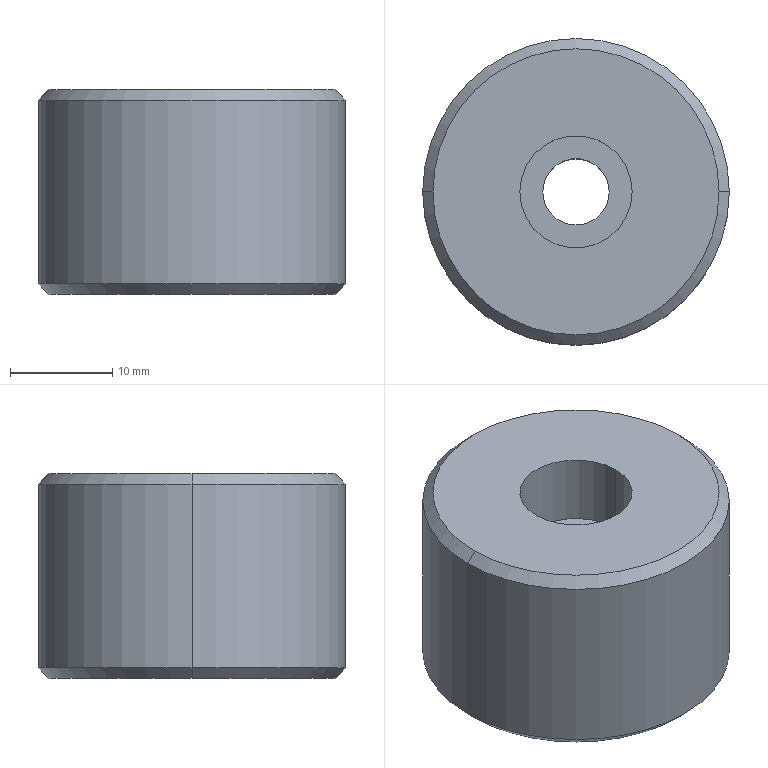Part | Creo | 1 solid | 13 faces | box 30 x 30 x 20 mm | volume 12948 mm3 | cylinder 6 | cone 4 | plane 3 | commonest cylinder face diameters 6.5 x2 11 x2 30 x2
STEP:
#1=CARTESIAN_POINT('',(-36.,235.,-210.5));
#2=VERTEX_POINT('',#1);
#3=CARTESIAN_POINT('',(-64.,235.,-210.5));
#4=VERTEX_POINT('',#3);
#5=CARTESIAN_POINT('',(-50.,235.,-210.5));
#6=DIRECTION('',(0.,0.,1.));
#7=DIRECTION('',(1.,0.,0.));
#8=AXIS2_PLACEMENT_3D('',#5,#6,#7);
#9=CIRCLE('',#8,14.);
#10=EDGE_CURVE('',#2,#4,#9,.T.);
#11=ORIENTED_EDGE('',*,*,#10,.F.);
#12=CARTESIAN_POINT('',(-50.,235.,-210.5));
#13=DIRECTION('',(0.,0.,1.));
#14=DIRECTION('',(-1.,0.,0.));
#15=AXIS2_PLACEMENT_3D('',#12,#13,#14);
#16=CIRCLE('',#15,14.);
#17=EDGE_CURVE('',#4,#2,#16,.T.);
#18=ORIENTED_EDGE('',*,*,#17,.F.);
#19=EDGE_LOOP('',(#11,#18));
#20=FACE_OUTER_BOUND('',#19,.F.);
#21=CARTESIAN_POINT('',(-55.5,235.,-210.5));
#22=VERTEX_POINT('',#21);
#23=CARTESIAN_POINT('',(-44.5,235.,-210.5));
#24=VERTEX_POINT('',#23);
#25=CARTESIAN_POINT('',(-50.,235.,-210.5));
#26=DIRECTION('',(0.,0.,-1.));
#27=DIRECTION('',(-1.,0.,0.));
#28=AXIS2_PLACEMENT_3D('',#25,#26,#27);
#29=CIRCLE('',#28,5.5);
#30=EDGE_CURVE('',#22,#24,#29,.T.);
#31=ORIENTED_EDGE('',*,*,#30,.F.);
#32=CARTESIAN_POINT('',(-50.,235.,-210.5));
#33=DIRECTION('',(0.,0.,-1.));
#34=DIRECTION('',(1.,0.,0.));
#35=AXIS2_PLACEMENT_3D('',#32,#33,#34);
#36=CIRCLE('',#35,5.5);
#37=EDGE_CURVE('',#24,#22,#36,.T.);
#38=ORIENTED_EDGE('',*,*,#37,.F.);
#39=EDGE_LOOP('',(#31,#38));
#40=FACE_BOUND('',#39,.F.);
#41=CARTESIAN_POINT('',(-50.,235.,-210.5));
#42=DIRECTION('',(0.,0.,1.));
#43=DIRECTION('',(1.,0.,0.));
#44=AXIS2_PLACEMENT_3D('',#41,#42,#43);
#45=PLANE('',#44);
#46=ADVANCED_FACE('',(#20,#40),#45,.T.);
#47=ORIENTED_EDGE('',*,*,#10,.T.);
#48=CARTESIAN_POINT('',(-65.,235.,-211.5));
#49=VERTEX_POINT('',#48);
#50=CARTESIAN_POINT('',(-64.,235.,-210.5));
#51=DIRECTION('',(-0.7071,0.,-0.7071));
#52=VECTOR('',#51,1.414);
#53=LINE('',#50,#52);
#54=EDGE_CURVE('',#4,#49,#53,.T.);
#55=ORIENTED_EDGE('',*,*,#54,.T.);
#56=CARTESIAN_POINT('',(-35.,235.,-211.5));
#57=VERTEX_POINT('',#56);
#58=CARTESIAN_POINT('',(-50.,235.,-211.5));
#59=DIRECTION('',(0.,0.,1.));
#60=DIRECTION('',(1.,0.,0.));
#61=AXIS2_PLACEMENT_3D('',#58,#59,#60);
#62=CIRCLE('',#61,15.);
#63=EDGE_CURVE('',#57,#49,#62,.T.);
#64=ORIENTED_EDGE('',*,*,#63,.F.);
#65=CARTESIAN_POINT('',(-36.,235.,-210.5));
#66=DIRECTION('',(0.7071,0.,-0.7071));
#67=VECTOR('',#66,1.414);
#68=LINE('',#65,#67);
#69=EDGE_CURVE('',#2,#57,#68,.T.);
#70=ORIENTED_EDGE('',*,*,#69,.F.);
#71=EDGE_LOOP('',(#47,#55,#64,#70));
#72=FACE_OUTER_BOUND('',#71,.F.);
#73=CARTESIAN_POINT('',(-50.,235.,-211.));
#74=DIRECTION('',(0.,0.,-1.));
#75=DIRECTION('',(-1.,0.,0.));
#76=AXIS2_PLACEMENT_3D('',#73,#74,#75);
#77=CONICAL_SURFACE('',#76,14.5,45.);
#78=ADVANCED_FACE('',(#72),#77,.T.);
#79=ORIENTED_EDGE('',*,*,#17,.T.);
#80=ORIENTED_EDGE('',*,*,#69,.T.);
#81=CARTESIAN_POINT('',(-50.,235.,-211.5));
#82=DIRECTION('',(0.,0.,1.));
#83=DIRECTION('',(-1.,0.,0.));
#84=AXIS2_PLACEMENT_3D('',#81,#82,#83);
#85=CIRCLE('',#84,15.);
#86=EDGE_CURVE('',#49,#57,#85,.T.);
#87=ORIENTED_EDGE('',*,*,#86,.F.);
#88=ORIENTED_EDGE('',*,*,#54,.F.);
#89=EDGE_LOOP('',(#79,#80,#87,#88));
#90=FACE_OUTER_BOUND('',#89,.F.);
#91=CARTESIAN_POINT('',(-50.,235.,-211.));
#92=DIRECTION('',(0.,0.,-1.));
#93=DIRECTION('',(-1.,0.,0.));
#94=AXIS2_PLACEMENT_3D('',#91,#92,#93);
#95=CONICAL_SURFACE('',#94,14.5,45.);
#96=ADVANCED_FACE('',(#90),#95,.T.);
#97=CARTESIAN_POINT('',(-35.,235.,-229.5));
#98=VERTEX_POINT('',#97);
#99=CARTESIAN_POINT('',(-65.,235.,-229.5));
#100=VERTEX_POINT('',#99);
#101=CARTESIAN_POINT('',(-50.,235.,-229.5));
#102=DIRECTION('',(0.,0.,-1.));
#103=DIRECTION('',(1.,0.,0.));
#104=AXIS2_PLACEMENT_3D('',#101,#102,#103);
#105=CIRCLE('',#104,15.);
#106=EDGE_CURVE('',#98,#100,#105,.T.);
#107=ORIENTED_EDGE('',*,*,#106,.T.);
#108=CARTESIAN_POINT('',(-65.,235.,-229.5));
#109=DIRECTION('',(0.,0.,1.));
#110=VECTOR('',#109,18.);
#111=LINE('',#108,#110);
#112=EDGE_CURVE('',#100,#49,#111,.T.);
#113=ORIENTED_EDGE('',*,*,#112,.T.);
#114=ORIENTED_EDGE('',*,*,#86,.T.);
#115=CARTESIAN_POINT('',(-35.,235.,-229.5));
#116=DIRECTION('',(0.,0.,1.));
#117=VECTOR('',#116,18.);
#118=LINE('',#115,#117);
#119=EDGE_CURVE('',#98,#57,#118,.T.);
#120=ORIENTED_EDGE('',*,*,#119,.F.);
#121=EDGE_LOOP('',(#107,#113,#114,#120));
#122=FACE_OUTER_BOUND('',#121,.F.);
#123=CARTESIAN_POINT('',(-50.,235.,-230.5));
#124=DIRECTION('',(0.,0.,1.));
#125=DIRECTION('',(1.,0.,0.));
#126=AXIS2_PLACEMENT_3D('',#123,#124,#125);
#127=CYLINDRICAL_SURFACE('',#126,15.);
#128=ADVANCED_FACE('',(#122),#127,.T.);
#129=CARTESIAN_POINT('',(-36.,235.,-230.5));
#130=VERTEX_POINT('',#129);
#131=CARTESIAN_POINT('',(-64.,235.,-230.5));
#132=VERTEX_POINT('',#131);
#133=CARTESIAN_POINT('',(-50.,235.,-230.5));
#134=DIRECTION('',(0.,0.,-1.));
#135=DIRECTION('',(1.,0.,0.));
#136=AXIS2_PLACEMENT_3D('',#133,#134,#135);
#137=CIRCLE('',#136,14.);
#138=EDGE_CURVE('',#130,#132,#137,.T.);
#139=ORIENTED_EDGE('',*,*,#138,.T.);
#140=CARTESIAN_POINT('',(-64.,235.,-230.5));
#141=DIRECTION('',(-0.7071,0.,0.7071));
#142=VECTOR('',#141,1.414);
#143=LINE('',#140,#142);
#144=EDGE_CURVE('',#132,#100,#143,.T.);
#145=ORIENTED_EDGE('',*,*,#144,.T.);
#146=ORIENTED_EDGE('',*,*,#106,.F.);
#147=CARTESIAN_POINT('',(-36.,235.,-230.5));
#148=DIRECTION('',(0.7071,0.,0.7071));
#149=VECTOR('',#148,1.414);
#150=LINE('',#147,#149);
#151=EDGE_CURVE('',#130,#98,#150,.T.);
#152=ORIENTED_EDGE('',*,*,#151,.F.);
#153=EDGE_LOOP('',(#139,#145,#146,#152));
#154=FACE_OUTER_BOUND('',#153,.F.);
#155=CARTESIAN_POINT('',(-50.,235.,-230.));
#156=DIRECTION('',(0.,0.,1.));
#157=DIRECTION('',(1.,0.,0.));
#158=AXIS2_PLACEMENT_3D('',#155,#156,#157);
#159=CONICAL_SURFACE('',#158,14.5,45.);
#160=ADVANCED_FACE('',(#154),#159,.T.);
#161=CARTESIAN_POINT('',(-50.,235.,-230.5));
#162=DIRECTION('',(0.,0.,-1.));
#163=DIRECTION('',(-1.,0.,0.));
#164=AXIS2_PLACEMENT_3D('',#161,#162,#163);
#165=CIRCLE('',#164,14.);
#166=EDGE_CURVE('',#132,#130,#165,.T.);
#167=ORIENTED_EDGE('',*,*,#166,.F.);
#168=ORIENTED_EDGE('',*,*,#138,.F.);
#169=EDGE_LOOP('',(#167,#168));
#170=FACE_OUTER_BOUND('',#169,.F.);
#171=CARTESIAN_POINT('',(-46.75,235.,-230.5));
#172=VERTEX_POINT('',#171);
#173=CARTESIAN_POINT('',(-53.25,235.,-230.5));
#174=VERTEX_POINT('',#173);
#175=CARTESIAN_POINT('',(-50.,235.,-230.5));
#176=DIRECTION('',(0.,0.,1.));
#177=DIRECTION('',(1.,0.,0.));
#178=AXIS2_PLACEMENT_3D('',#175,#176,#177);
#179=CIRCLE('',#178,3.25);
#180=EDGE_CURVE('',#172,#174,#179,.T.);
#181=ORIENTED_EDGE('',*,*,#180,.F.);
#182=CARTESIAN_POINT('',(-50.,235.,-230.5));
#183=DIRECTION('',(0.,0.,1.));
#184=DIRECTION('',(-1.,0.,0.));
#185=AXIS2_PLACEMENT_3D('',#182,#183,#184);
#186=CIRCLE('',#185,3.25);
#187=EDGE_CURVE('',#174,#172,#186,.T.);
#188=ORIENTED_EDGE('',*,*,#187,.F.);
#189=EDGE_LOOP('',(#181,#188));
#190=FACE_BOUND('',#189,.F.);
#191=CARTESIAN_POINT('',(-50.,235.,-230.5));
#192=DIRECTION('',(0.,0.,-1.));
#193=DIRECTION('',(-1.,0.,0.));
#194=AXIS2_PLACEMENT_3D('',#191,#192,#193);
#195=PLANE('',#194);
#196=ADVANCED_FACE('',(#170,#190),#195,.T.);
#197=ORIENTED_EDGE('',*,*,#166,.T.);
#198=ORIENTED_EDGE('',*,*,#151,.T.);
#199=CARTESIAN_POINT('',(-50.,235.,-229.5));
#200=DIRECTION('',(0.,0.,-1.));
#201=DIRECTION('',(-1.,0.,0.));
#202=AXIS2_PLACEMENT_3D('',#199,#200,#201);
#203=CIRCLE('',#202,15.);
#204=EDGE_CURVE('',#100,#98,#203,.T.);
#205=ORIENTED_EDGE('',*,*,#204,.F.);
#206=ORIENTED_EDGE('',*,*,#144,.F.);
#207=EDGE_LOOP('',(#197,#198,#205,#206));
#208=FACE_OUTER_BOUND('',#207,.F.);
#209=CARTESIAN_POINT('',(-50.,235.,-230.));
#210=DIRECTION('',(0.,0.,1.));
#211=DIRECTION('',(1.,0.,0.));
#212=AXIS2_PLACEMENT_3D('',#209,#210,#211);
#213=CONICAL_SURFACE('',#212,14.5,45.);
#214=ADVANCED_FACE('',(#208),#213,.T.);
#215=ORIENTED_EDGE('',*,*,#204,.T.);
#216=ORIENTED_EDGE('',*,*,#119,.T.);
#217=ORIENTED_EDGE('',*,*,#63,.T.);
#218=ORIENTED_EDGE('',*,*,#112,.F.);
#219=EDGE_LOOP('',(#215,#216,#217,#218));
#220=FACE_OUTER_BOUND('',#219,.F.);
#221=CARTESIAN_POINT('',(-50.,235.,-230.5));
#222=DIRECTION('',(0.,0.,1.));
#223=DIRECTION('',(1.,0.,0.));
#224=AXIS2_PLACEMENT_3D('',#221,#222,#223);
#225=CYLINDRICAL_SURFACE('',#224,15.);
#226=ADVANCED_FACE('',(#220),#225,.T.);
#227=CARTESIAN_POINT('',(-53.25,235.,-217.5));
#228=VERTEX_POINT('',#227);
#229=CARTESIAN_POINT('',(-46.75,235.,-217.5));
#230=VERTEX_POINT('',#229);
#231=CARTESIAN_POINT('',(-50.,235.,-217.5));
#232=DIRECTION('',(0.,0.,-1.));
#233=DIRECTION('',(-1.,0.,0.));
#234=AXIS2_PLACEMENT_3D('',#231,#232,#233);
#235=CIRCLE('',#234,3.25);
#236=EDGE_CURVE('',#228,#230,#235,.T.);
#237=ORIENTED_EDGE('',*,*,#236,.T.);
#238=CARTESIAN_POINT('',(-46.75,235.,-217.5));
#239=DIRECTION('',(0.,0.,-1.));
#240=VECTOR('',#239,13.);
#241=LINE('',#238,#240);
#242=EDGE_CURVE('',#230,#172,#241,.T.);
#243=ORIENTED_EDGE('',*,*,#242,.T.);
#244=ORIENTED_EDGE('',*,*,#180,.T.);
#245=CARTESIAN_POINT('',(-53.25,235.,-217.5));
#246=DIRECTION('',(0.,0.,-1.));
#247=VECTOR('',#246,13.);
#248=LINE('',#245,#247);
#249=EDGE_CURVE('',#228,#174,#248,.T.);
#250=ORIENTED_EDGE('',*,*,#249,.F.);
#251=EDGE_LOOP('',(#237,#243,#244,#250));
#252=FACE_OUTER_BOUND('',#251,.F.);
#253=CARTESIAN_POINT('',(-50.,235.,-210.5));
#254=DIRECTION('',(0.,0.,-1.));
#255=DIRECTION('',(-1.,0.,0.));
#256=AXIS2_PLACEMENT_3D('',#253,#254,#255);
#257=CYLINDRICAL_SURFACE('',#256,3.25);
#258=ADVANCED_FACE('',(#252),#257,.F.);
#259=CARTESIAN_POINT('',(-44.5,235.,-217.5));
#260=VERTEX_POINT('',#259);
#261=CARTESIAN_POINT('',(-55.5,235.,-217.5));
#262=VERTEX_POINT('',#261);
#263=CARTESIAN_POINT('',(-50.,235.,-217.5));
#264=DIRECTION('',(0.,0.,1.));
#265=DIRECTION('',(1.,0.,0.));
#266=AXIS2_PLACEMENT_3D('',#263,#264,#265);
#267=CIRCLE('',#266,5.5);
#268=EDGE_CURVE('',#260,#262,#267,.T.);
#269=ORIENTED_EDGE('',*,*,#268,.F.);
#270=CARTESIAN_POINT('',(-50.,235.,-217.5));
#271=DIRECTION('',(0.,0.,1.));
#272=DIRECTION('',(-1.,0.,0.));
#273=AXIS2_PLACEMENT_3D('',#270,#271,#272);
#274=CIRCLE('',#273,5.5);
#275=EDGE_CURVE('',#262,#260,#274,.T.);
#276=ORIENTED_EDGE('',*,*,#275,.F.);
#277=EDGE_LOOP('',(#269,#276));
#278=FACE_OUTER_BOUND('',#277,.F.);
#279=ORIENTED_EDGE('',*,*,#236,.F.);
#280=CARTESIAN_POINT('',(-50.,235.,-217.5));
#281=DIRECTION('',(0.,0.,-1.));
#282=DIRECTION('',(1.,0.,0.));
#283=AXIS2_PLACEMENT_3D('',#280,#281,#282);
#284=CIRCLE('',#283,3.25);
#285=EDGE_CURVE('',#230,#228,#284,.T.);
#286=ORIENTED_EDGE('',*,*,#285,.F.);
#287=EDGE_LOOP('',(#279,#286));
#288=FACE_BOUND('',#287,.F.);
#289=CARTESIAN_POINT('',(-50.,235.,-217.5));
#290=DIRECTION('',(0.,0.,-1.));
#291=DIRECTION('',(-1.,0.,0.));
#292=AXIS2_PLACEMENT_3D('',#289,#290,#291);
#293=PLANE('',#292);
#294=ADVANCED_FACE('',(#278,#288),#293,.F.);
#295=ORIENTED_EDGE('',*,*,#268,.T.);
#296=CARTESIAN_POINT('',(-55.5,235.,-210.5));
#297=DIRECTION('',(0.,0.,-1.));
#298=VECTOR('',#297,7.);
#299=LINE('',#296,#298);
#300=EDGE_CURVE('',#22,#262,#299,.T.);
#301=ORIENTED_EDGE('',*,*,#300,.F.);
#302=ORIENTED_EDGE('',*,*,#30,.T.);
#303=CARTESIAN_POINT('',(-44.5,235.,-210.5));
#304=DIRECTION('',(0.,0.,-1.));
#305=VECTOR('',#304,7.);
#306=LINE('',#303,#305);
#307=EDGE_CURVE('',#24,#260,#306,.T.);
#308=ORIENTED_EDGE('',*,*,#307,.T.);
#309=EDGE_LOOP('',(#295,#301,#302,#308));
#310=FACE_OUTER_BOUND('',#309,.F.);
#311=CARTESIAN_POINT('',(-50.,235.,-210.5));
#312=DIRECTION('',(0.,0.,-1.));
#313=DIRECTION('',(-1.,0.,0.));
#314=AXIS2_PLACEMENT_3D('',#311,#312,#313);
#315=CYLINDRICAL_SURFACE('',#314,5.5);
#316=ADVANCED_FACE('',(#310),#315,.F.);
#317=ORIENTED_EDGE('',*,*,#275,.T.);
#318=ORIENTED_EDGE('',*,*,#307,.F.);
#319=ORIENTED_EDGE('',*,*,#37,.T.);
#320=ORIENTED_EDGE('',*,*,#300,.T.);
#321=EDGE_LOOP('',(#317,#318,#319,#320));
#322=FACE_OUTER_BOUND('',#321,.F.);
#323=CARTESIAN_POINT('',(-50.,235.,-210.5));
#324=DIRECTION('',(0.,0.,-1.));
#325=DIRECTION('',(-1.,0.,0.));
#326=AXIS2_PLACEMENT_3D('',#323,#324,#325);
#327=CYLINDRICAL_SURFACE('',#326,5.5);
#328=ADVANCED_FACE('',(#322),#327,.F.);
#329=ORIENTED_EDGE('',*,*,#285,.T.);
#330=ORIENTED_EDGE('',*,*,#249,.T.);
#331=ORIENTED_EDGE('',*,*,#187,.T.);
#332=ORIENTED_EDGE('',*,*,#242,.F.);
#333=EDGE_LOOP('',(#329,#330,#331,#332));
#334=FACE_OUTER_BOUND('',#333,.F.);
#335=CARTESIAN_POINT('',(-50.,235.,-210.5));
#336=DIRECTION('',(0.,0.,-1.));
#337=DIRECTION('',(-1.,0.,0.));
#338=AXIS2_PLACEMENT_3D('',#335,#336,#337);
#339=CYLINDRICAL_SURFACE('',#338,3.25);
#340=ADVANCED_FACE('',(#334),#339,.F.);
#341=CLOSED_SHELL('',(#46,#78,#96,#128,#160,#196,#214,#226,#258,#294,#316,#328,#340));
#342=MANIFOLD_SOLID_BREP('',#341);
#343=(LENGTH_UNIT()NAMED_UNIT(*)SI_UNIT(.MILLI.,.METRE.));
#344=UNCERTAINTY_MEASURE_WITH_UNIT(LENGTH_MEASURE(0.00469),#343,'','');
#345=(NAMED_UNIT(*)PLANE_ANGLE_UNIT()SI_UNIT($,.RADIAN.));
#346=PLANE_ANGLE_MEASURE_WITH_UNIT(PLANE_ANGLE_MEASURE(0.01745),#345);
#347=(CONVERSION_BASED_UNIT('DEGREE',#346)NAMED_UNIT(*)PLANE_ANGLE_UNIT());
#348=(NAMED_UNIT(*)SI_UNIT($,.STERADIAN.)SOLID_ANGLE_UNIT());
#349=(GEOMETRIC_REPRESENTATION_CONTEXT(3)GLOBAL_UNCERTAINTY_ASSIGNED_CONTEXT((#344))GLOBAL_UNIT_ASSIGNED_CONTEXT((#343,#347,#348))REPRESENTATION_CONTEXT('',''));
#350=ADVANCED_BREP_SHAPE_REPRESENTATION('',(#342),#349);